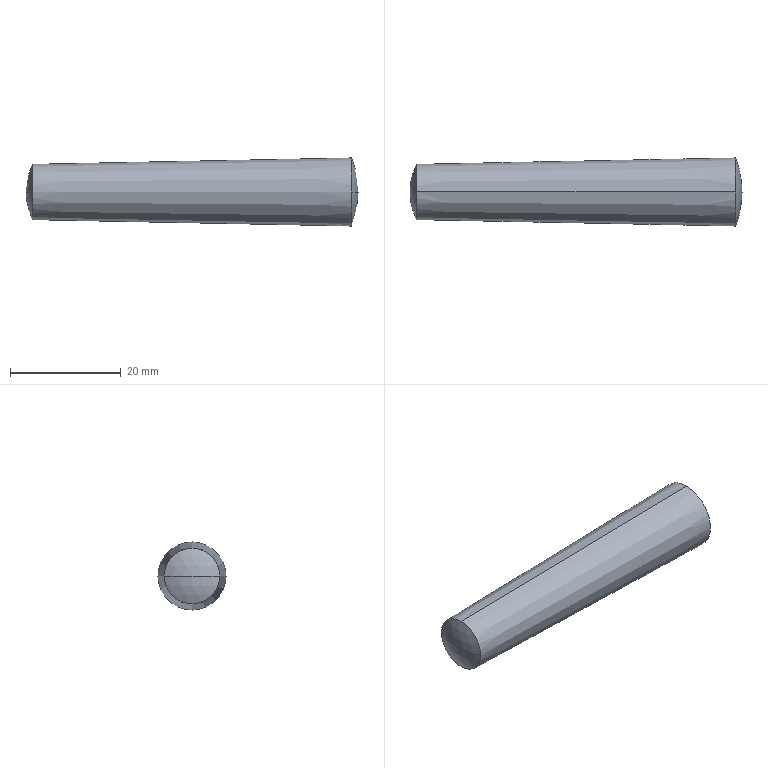Part | SolidWorks | features Revolution 1 | 1 solid | 6 faces | box 60 x 12.304 x 12.304 mm | volume 5767 mm3 | sphere 4 | cone 2
STEP:
#1=CARTESIAN_POINT('',(1.2,0.,5.));
#2=VERTEX_POINT('',#1);
#3=CARTESIAN_POINT('',(1.2,5.,0.));
#4=VERTEX_POINT('',#3);
#5=CARTESIAN_POINT('',(1.2,0.,0.));
#6=DIRECTION('',(-1.,0.,0.));
#7=DIRECTION('',(0.,0.,1.));
#8=AXIS2_PLACEMENT_3D('',#5,#6,#7);
#9=CIRCLE('',#8,5.);
#10=EDGE_CURVE('',#2,#4,#9,.T.);
#11=ORIENTED_EDGE('',*,*,#10,.F.);
#12=CARTESIAN_POINT('',(58.8,0.,6.152));
#13=VERTEX_POINT('',#12);
#14=CARTESIAN_POINT('',(58.8,0.,6.152));
#15=DIRECTION('',(0.9998,0.,0.02));
#16=VECTOR('',#15,1000.);
#17=LINE('',#14,#16);
#18=EDGE_CURVE('',#2,#13,#17,.T.);
#19=ORIENTED_EDGE('',*,*,#18,.T.);
#20=CARTESIAN_POINT('',(58.8,6.152,0.));
#21=VERTEX_POINT('',#20);
#22=CARTESIAN_POINT('',(58.8,0.,0.));
#23=DIRECTION('',(-1.,0.,0.));
#24=DIRECTION('',(0.,0.,1.));
#25=AXIS2_PLACEMENT_3D('',#22,#23,#24);
#26=CIRCLE('',#25,6.152);
#27=EDGE_CURVE('',#13,#21,#26,.T.);
#28=ORIENTED_EDGE('',*,*,#27,.T.);
#29=CARTESIAN_POINT('',(58.8,0.,-6.152));
#30=VERTEX_POINT('',#29);
#31=CARTESIAN_POINT('',(58.8,0.,0.));
#32=DIRECTION('',(-1.,0.,0.));
#33=DIRECTION('',(0.,0.,1.));
#34=AXIS2_PLACEMENT_3D('',#31,#32,#33);
#35=CIRCLE('',#34,6.152);
#36=EDGE_CURVE('',#21,#30,#35,.T.);
#37=ORIENTED_EDGE('',*,*,#36,.T.);
#38=CARTESIAN_POINT('',(1.2,0.,-5.));
#39=VERTEX_POINT('',#38);
#40=CARTESIAN_POINT('',(58.8,0.,-6.152));
#41=DIRECTION('',(0.9998,0.,-0.02));
#42=VECTOR('',#41,1000.);
#43=LINE('',#40,#42);
#44=EDGE_CURVE('',#39,#30,#43,.T.);
#45=ORIENTED_EDGE('',*,*,#44,.F.);
#46=CARTESIAN_POINT('',(1.2,0.,0.));
#47=DIRECTION('',(-1.,0.,0.));
#48=DIRECTION('',(0.,0.,1.));
#49=AXIS2_PLACEMENT_3D('',#46,#47,#48);
#50=CIRCLE('',#49,5.);
#51=EDGE_CURVE('',#4,#39,#50,.T.);
#52=ORIENTED_EDGE('',*,*,#51,.F.);
#53=EDGE_LOOP('',(#11,#19,#28,#37,#45,#52));
#54=FACE_OUTER_BOUND('',#53,.T.);
#55=CARTESIAN_POINT('',(58.8,0.,0.));
#56=DIRECTION('',(1.,0.,0.));
#57=DIRECTION('',(0.,0.,-1.));
#58=AXIS2_PLACEMENT_3D('',#55,#56,#57);
#59=CONICAL_SURFACE('',#58,6.152,0.02);
#60=ADVANCED_FACE('',(#54),#59,.T.);
#61=CARTESIAN_POINT('',(60.,0.,0.));
#62=VERTEX_POINT('',#61);
#63=CARTESIAN_POINT('',(43.63,0.,0.));
#64=DIRECTION('',(0.,0.,1.));
#65=DIRECTION('',(1.,0.,0.));
#66=AXIS2_PLACEMENT_3D('',#63,#64,#65);
#67=CIRCLE('',#66,16.37);
#68=EDGE_CURVE('',#62,#21,#67,.T.);
#69=ORIENTED_EDGE('',*,*,#68,.F.);
#70=CARTESIAN_POINT('',(58.8,-6.152,0.));
#71=VERTEX_POINT('',#70);
#72=CARTESIAN_POINT('',(43.63,0.,0.));
#73=DIRECTION('',(0.,0.,-1.));
#74=DIRECTION('',(0.,1.,0.));
#75=AXIS2_PLACEMENT_3D('',#72,#73,#74);
#76=CIRCLE('',#75,16.37);
#77=EDGE_CURVE('',#62,#71,#76,.T.);
#78=ORIENTED_EDGE('',*,*,#77,.T.);
#79=CARTESIAN_POINT('',(58.8,0.,0.));
#80=DIRECTION('',(-1.,0.,0.));
#81=DIRECTION('',(0.,0.,1.));
#82=AXIS2_PLACEMENT_3D('',#79,#80,#81);
#83=CIRCLE('',#82,6.152);
#84=EDGE_CURVE('',#30,#71,#83,.T.);
#85=ORIENTED_EDGE('',*,*,#84,.F.);
#86=ORIENTED_EDGE('',*,*,#36,.F.);
#87=EDGE_LOOP('',(#69,#78,#85,#86));
#88=FACE_OUTER_BOUND('',#87,.T.);
#89=CARTESIAN_POINT('',(43.63,0.,0.));
#90=DIRECTION('',(0.,0.,-1.));
#91=DIRECTION('',(0.,1.,0.));
#92=AXIS2_PLACEMENT_3D('',#89,#90,#91);
#93=SPHERICAL_SURFACE('',#92,16.37);
#94=ADVANCED_FACE('',(#88),#93,.T.);
#95=ORIENTED_EDGE('',*,*,#51,.T.);
#96=CARTESIAN_POINT('',(1.2,-5.,0.));
#97=VERTEX_POINT('',#96);
#98=CARTESIAN_POINT('',(1.2,0.,0.));
#99=DIRECTION('',(-1.,0.,0.));
#100=DIRECTION('',(0.,0.,1.));
#101=AXIS2_PLACEMENT_3D('',#98,#99,#100);
#102=CIRCLE('',#101,5.);
#103=EDGE_CURVE('',#39,#97,#102,.T.);
#104=ORIENTED_EDGE('',*,*,#103,.T.);
#105=CARTESIAN_POINT('',(0.,0.,0.));
#106=VERTEX_POINT('',#105);
#107=CARTESIAN_POINT('',(11.017,0.,0.));
#108=DIRECTION('',(0.,0.,-1.));
#109=DIRECTION('',(0.,1.,0.));
#110=AXIS2_PLACEMENT_3D('',#107,#108,#109);
#111=CIRCLE('',#110,11.017);
#112=EDGE_CURVE('',#97,#106,#111,.T.);
#113=ORIENTED_EDGE('',*,*,#112,.T.);
#114=CARTESIAN_POINT('',(11.017,0.,0.));
#115=DIRECTION('',(0.,0.,1.));
#116=DIRECTION('',(1.,0.,0.));
#117=AXIS2_PLACEMENT_3D('',#114,#115,#116);
#118=CIRCLE('',#117,11.017);
#119=EDGE_CURVE('',#4,#106,#118,.T.);
#120=ORIENTED_EDGE('',*,*,#119,.F.);
#121=EDGE_LOOP('',(#95,#104,#113,#120));
#122=FACE_OUTER_BOUND('',#121,.T.);
#123=CARTESIAN_POINT('',(11.017,0.,0.));
#124=DIRECTION('',(0.,0.,-1.));
#125=DIRECTION('',(0.,1.,0.));
#126=AXIS2_PLACEMENT_3D('',#123,#124,#125);
#127=SPHERICAL_SURFACE('',#126,11.017);
#128=ADVANCED_FACE('',(#122),#127,.T.);
#129=ORIENTED_EDGE('',*,*,#112,.F.);
#130=CARTESIAN_POINT('',(1.2,0.,0.));
#131=DIRECTION('',(-1.,0.,0.));
#132=DIRECTION('',(0.,0.,1.));
#133=AXIS2_PLACEMENT_3D('',#130,#131,#132);
#134=CIRCLE('',#133,5.);
#135=EDGE_CURVE('',#97,#2,#134,.T.);
#136=ORIENTED_EDGE('',*,*,#135,.T.);
#137=ORIENTED_EDGE('',*,*,#10,.T.);
#138=ORIENTED_EDGE('',*,*,#119,.T.);
#139=EDGE_LOOP('',(#129,#136,#137,#138));
#140=FACE_OUTER_BOUND('',#139,.T.);
#141=CARTESIAN_POINT('',(11.017,0.,0.));
#142=DIRECTION('',(0.,0.,-1.));
#143=DIRECTION('',(0.,1.,0.));
#144=AXIS2_PLACEMENT_3D('',#141,#142,#143);
#145=SPHERICAL_SURFACE('',#144,11.017);
#146=ADVANCED_FACE('',(#140),#145,.T.);
#147=ORIENTED_EDGE('',*,*,#77,.F.);
#148=ORIENTED_EDGE('',*,*,#68,.T.);
#149=ORIENTED_EDGE('',*,*,#27,.F.);
#150=CARTESIAN_POINT('',(58.8,0.,0.));
#151=DIRECTION('',(-1.,0.,0.));
#152=DIRECTION('',(0.,0.,1.));
#153=AXIS2_PLACEMENT_3D('',#150,#151,#152);
#154=CIRCLE('',#153,6.152);
#155=EDGE_CURVE('',#71,#13,#154,.T.);
#156=ORIENTED_EDGE('',*,*,#155,.F.);
#157=EDGE_LOOP('',(#147,#148,#149,#156));
#158=FACE_OUTER_BOUND('',#157,.T.);
#159=CARTESIAN_POINT('',(43.63,0.,0.));
#160=DIRECTION('',(0.,0.,-1.));
#161=DIRECTION('',(0.,1.,0.));
#162=AXIS2_PLACEMENT_3D('',#159,#160,#161);
#163=SPHERICAL_SURFACE('',#162,16.37);
#164=ADVANCED_FACE('',(#158),#163,.T.);
#165=ORIENTED_EDGE('',*,*,#18,.F.);
#166=ORIENTED_EDGE('',*,*,#135,.F.);
#167=ORIENTED_EDGE('',*,*,#103,.F.);
#168=ORIENTED_EDGE('',*,*,#44,.T.);
#169=ORIENTED_EDGE('',*,*,#84,.T.);
#170=ORIENTED_EDGE('',*,*,#155,.T.);
#171=EDGE_LOOP('',(#165,#166,#167,#168,#169,#170));
#172=FACE_OUTER_BOUND('',#171,.T.);
#173=CARTESIAN_POINT('',(58.8,0.,0.));
#174=DIRECTION('',(1.,0.,0.));
#175=DIRECTION('',(0.,0.,-1.));
#176=AXIS2_PLACEMENT_3D('',#173,#174,#175);
#177=CONICAL_SURFACE('',#176,6.152,0.02);
#178=ADVANCED_FACE('',(#172),#177,.T.);
#179=CLOSED_SHELL('',(#60,#94,#128,#146,#164,#178));
#180=MANIFOLD_SOLID_BREP('',#179);
#181=CARTESIAN_POINT('',(0.,0.,0.));
#182=DIRECTION('',(0.,0.,1.));
#183=DIRECTION('',(1.,0.,0.));
#184=AXIS2_PLACEMENT_3D('',#181,#182,#183);
#185=(LENGTH_UNIT()NAMED_UNIT(*)SI_UNIT(.MILLI.,.METRE.));
#186=UNCERTAINTY_MEASURE_WITH_UNIT(LENGTH_MEASURE(0.00001),#185,'','');
#187=(NAMED_UNIT(*)PLANE_ANGLE_UNIT()SI_UNIT($,.RADIAN.));
#188=(NAMED_UNIT(*)SI_UNIT($,.STERADIAN.)SOLID_ANGLE_UNIT());
#189=(GEOMETRIC_REPRESENTATION_CONTEXT(3)GLOBAL_UNCERTAINTY_ASSIGNED_CONTEXT((#186))GLOBAL_UNIT_ASSIGNED_CONTEXT((#185,#187,#188))REPRESENTATION_CONTEXT('',''));
#190=ADVANCED_BREP_SHAPE_REPRESENTATION('',(#180,#184),#189);